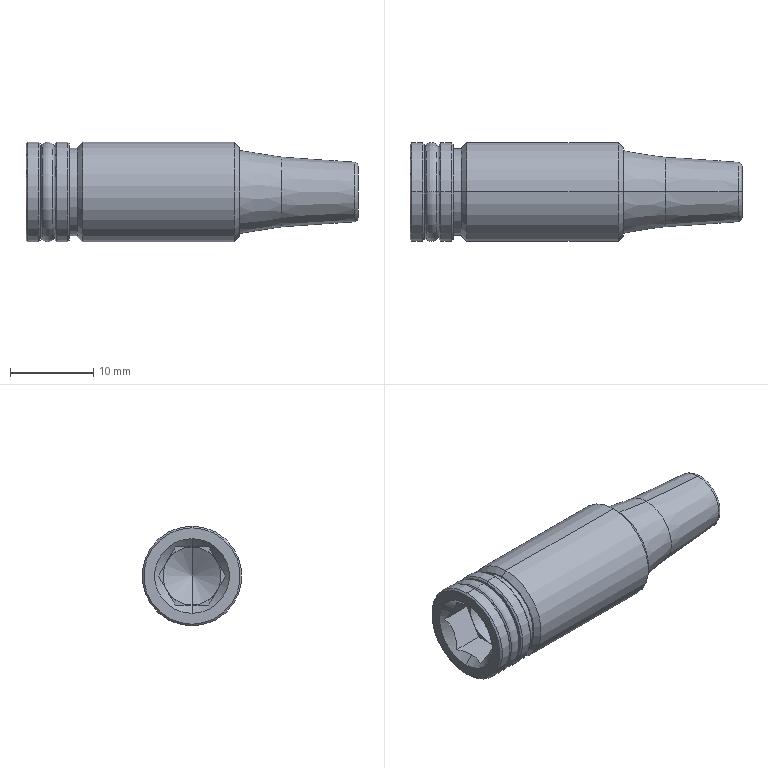Part | STEP file | 160_C_Screw | 1 solid | 68 faces | box 40 x 12 x 12 mm | volume 3167 mm3 | cone 20 | plane 20 | cylinder 16 | torus 12 | commonest cylinder face diameters 12 x6 9.5 x4 7 x2 8 x2 10.5 x2